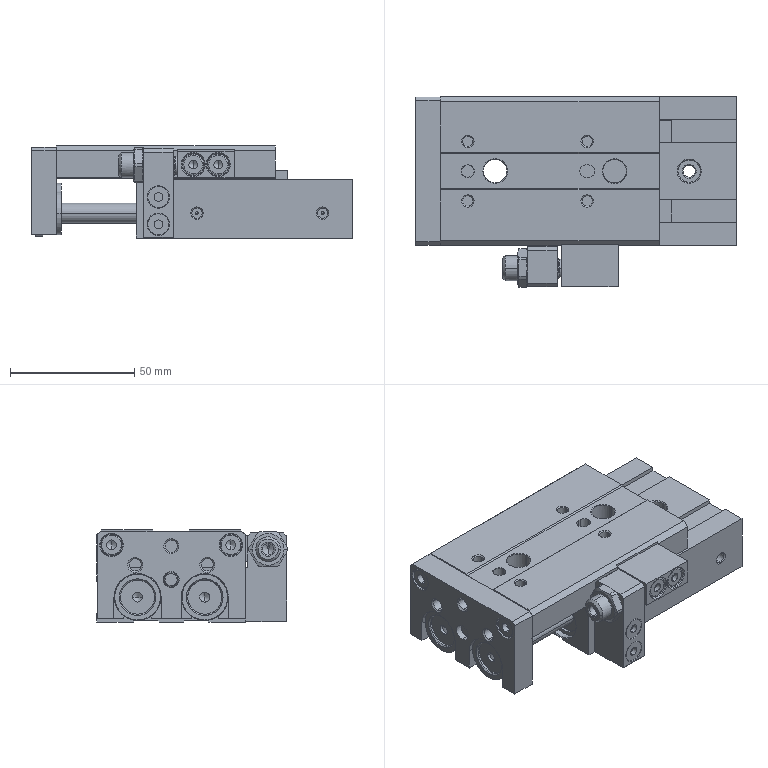Part | SolidWorks | 3 solids | 565 faces | box 129 x 76.75 x 37 mm | volume 182069 mm3 | plane 240 | cylinder 197 | cone 114 | spline 14 | commonest cylinder face diameters 4.134 x28 9 x20 8.5 x12 4 x11 4.917 x10 5 x10